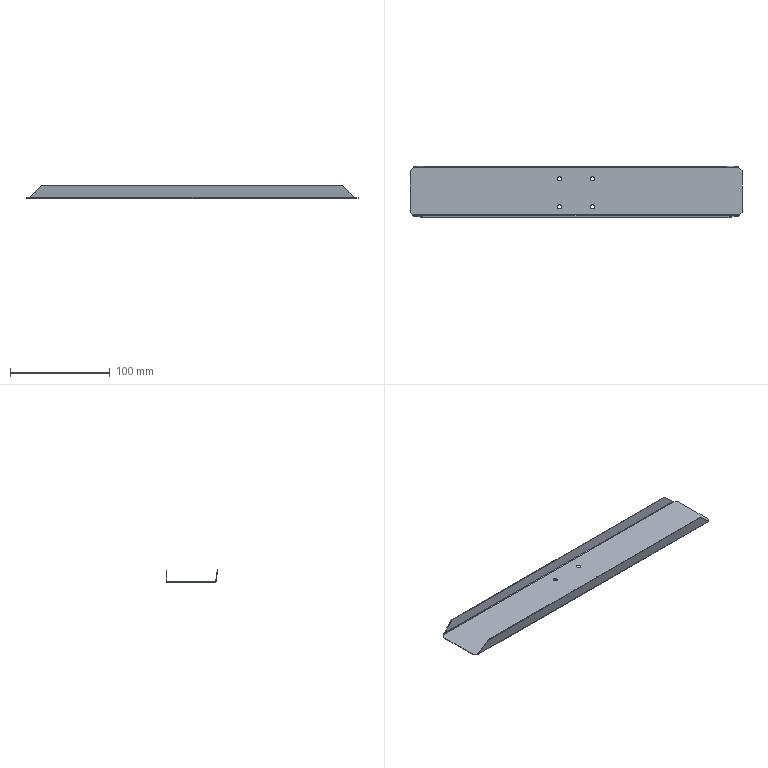Part | SolidWorks | features BaseBody 1 | 1 solid | 34 faces | box 332.2 x 51.676 x 12.864 mm | volume 11858 mm3 | plane 18 | cylinder 12 | spline 4 | commonest cylinder face diameters 4.17 x8 1.5 x2 2.5 x2
STEP:
#1=CARTESIAN_POINT('',(-18.585,-15.223,0.));
#2=VERTEX_POINT('',#1);
#3=CARTESIAN_POINT('',(-14.415,-15.223,0.));
#4=VERTEX_POINT('',#3);
#5=CARTESIAN_POINT('',(-16.5,-15.223,0.));
#6=DIRECTION('',(0.,0.,1.));
#7=DIRECTION('',(-1.,0.,0.));
#8=AXIS2_PLACEMENT_3D('',#5,#6,#7);
#9=CIRCLE('',#8,2.085);
#10=EDGE_CURVE('',#2,#4,#9,.T.);
#11=ORIENTED_EDGE('',*,*,#10,.T.);
#12=CARTESIAN_POINT('',(-14.415,-15.223,-0.5));
#13=VERTEX_POINT('',#12);
#14=CARTESIAN_POINT('',(-14.415,-15.223,0.));
#15=DIRECTION('',(0.,0.,-1.));
#16=VECTOR('',#15,1000.);
#17=LINE('',#14,#16);
#18=EDGE_CURVE('',#4,#13,#17,.T.);
#19=ORIENTED_EDGE('',*,*,#18,.T.);
#20=CARTESIAN_POINT('',(-18.585,-15.223,-0.5));
#21=VERTEX_POINT('',#20);
#22=CARTESIAN_POINT('',(-16.5,-15.223,-0.5));
#23=DIRECTION('',(0.,0.,-1.));
#24=DIRECTION('',(-1.,0.,0.));
#25=AXIS2_PLACEMENT_3D('',#22,#23,#24);
#26=CIRCLE('',#25,2.085);
#27=EDGE_CURVE('',#13,#21,#26,.T.);
#28=ORIENTED_EDGE('',*,*,#27,.T.);
#29=CARTESIAN_POINT('',(-18.585,-15.223,0.));
#30=DIRECTION('',(0.,0.,-1.));
#31=VECTOR('',#30,1000.);
#32=LINE('',#29,#31);
#33=EDGE_CURVE('',#2,#21,#32,.T.);
#34=ORIENTED_EDGE('',*,*,#33,.F.);
#35=EDGE_LOOP('',(#11,#19,#28,#34));
#36=FACE_OUTER_BOUND('',#35,.T.);
#37=CARTESIAN_POINT('',(-16.5,-15.223,0.));
#38=DIRECTION('',(0.,0.,-1.));
#39=DIRECTION('',(-1.,0.,0.));
#40=AXIS2_PLACEMENT_3D('',#37,#38,#39);
#41=CYLINDRICAL_SURFACE('',#40,2.085);
#42=ADVANCED_FACE('',(#36),#41,.F.);
#43=CARTESIAN_POINT('',(14.415,12.777,0.));
#44=VERTEX_POINT('',#43);
#45=CARTESIAN_POINT('',(18.585,12.777,0.));
#46=VERTEX_POINT('',#45);
#47=CARTESIAN_POINT('',(16.5,12.777,0.));
#48=DIRECTION('',(0.,0.,1.));
#49=DIRECTION('',(-1.,0.,0.));
#50=AXIS2_PLACEMENT_3D('',#47,#48,#49);
#51=CIRCLE('',#50,2.085);
#52=EDGE_CURVE('',#44,#46,#51,.T.);
#53=ORIENTED_EDGE('',*,*,#52,.T.);
#54=CARTESIAN_POINT('',(18.585,12.777,-0.5));
#55=VERTEX_POINT('',#54);
#56=CARTESIAN_POINT('',(18.585,12.777,0.));
#57=DIRECTION('',(0.,0.,-1.));
#58=VECTOR('',#57,1000.);
#59=LINE('',#56,#58);
#60=EDGE_CURVE('',#46,#55,#59,.T.);
#61=ORIENTED_EDGE('',*,*,#60,.T.);
#62=CARTESIAN_POINT('',(14.415,12.777,-0.5));
#63=VERTEX_POINT('',#62);
#64=CARTESIAN_POINT('',(16.5,12.777,-0.5));
#65=DIRECTION('',(0.,0.,1.));
#66=DIRECTION('',(-1.,0.,0.));
#67=AXIS2_PLACEMENT_3D('',#64,#65,#66);
#68=CIRCLE('',#67,2.085);
#69=EDGE_CURVE('',#63,#55,#68,.T.);
#70=ORIENTED_EDGE('',*,*,#69,.F.);
#71=CARTESIAN_POINT('',(14.415,12.777,0.));
#72=DIRECTION('',(0.,0.,-1.));
#73=VECTOR('',#72,1000.);
#74=LINE('',#71,#73);
#75=EDGE_CURVE('',#44,#63,#74,.T.);
#76=ORIENTED_EDGE('',*,*,#75,.F.);
#77=EDGE_LOOP('',(#53,#61,#70,#76));
#78=FACE_OUTER_BOUND('',#77,.T.);
#79=CARTESIAN_POINT('',(16.5,12.777,0.));
#80=DIRECTION('',(0.,0.,-1.));
#81=DIRECTION('',(-1.,0.,0.));
#82=AXIS2_PLACEMENT_3D('',#79,#80,#81);
#83=CYLINDRICAL_SURFACE('',#82,2.085);
#84=ADVANCED_FACE('',(#78),#83,.F.);
#85=CARTESIAN_POINT('',(-18.585,12.777,0.));
#86=VERTEX_POINT('',#85);
#87=CARTESIAN_POINT('',(-14.415,12.777,0.));
#88=VERTEX_POINT('',#87);
#89=CARTESIAN_POINT('',(-16.5,12.777,0.));
#90=DIRECTION('',(0.,0.,1.));
#91=DIRECTION('',(-1.,0.,0.));
#92=AXIS2_PLACEMENT_3D('',#89,#90,#91);
#93=CIRCLE('',#92,2.085);
#94=EDGE_CURVE('',#86,#88,#93,.T.);
#95=ORIENTED_EDGE('',*,*,#94,.T.);
#96=CARTESIAN_POINT('',(-14.415,12.777,-0.5));
#97=VERTEX_POINT('',#96);
#98=CARTESIAN_POINT('',(-14.415,12.777,0.));
#99=DIRECTION('',(0.,0.,-1.));
#100=VECTOR('',#99,1000.);
#101=LINE('',#98,#100);
#102=EDGE_CURVE('',#88,#97,#101,.T.);
#103=ORIENTED_EDGE('',*,*,#102,.T.);
#104=CARTESIAN_POINT('',(-18.585,12.777,-0.5));
#105=VERTEX_POINT('',#104);
#106=CARTESIAN_POINT('',(-16.5,12.777,-0.5));
#107=DIRECTION('',(0.,0.,1.));
#108=DIRECTION('',(-1.,0.,0.));
#109=AXIS2_PLACEMENT_3D('',#106,#107,#108);
#110=CIRCLE('',#109,2.085);
#111=EDGE_CURVE('',#105,#97,#110,.T.);
#112=ORIENTED_EDGE('',*,*,#111,.F.);
#113=CARTESIAN_POINT('',(-18.585,12.777,0.));
#114=DIRECTION('',(0.,0.,-1.));
#115=VECTOR('',#114,1000.);
#116=LINE('',#113,#115);
#117=EDGE_CURVE('',#86,#105,#116,.T.);
#118=ORIENTED_EDGE('',*,*,#117,.F.);
#119=EDGE_LOOP('',(#95,#103,#112,#118));
#120=FACE_OUTER_BOUND('',#119,.T.);
#121=CARTESIAN_POINT('',(-16.5,12.777,0.));
#122=DIRECTION('',(0.,0.,-1.));
#123=DIRECTION('',(-1.,0.,0.));
#124=AXIS2_PLACEMENT_3D('',#121,#122,#123);
#125=CYLINDRICAL_SURFACE('',#124,2.085);
#126=ADVANCED_FACE('',(#120),#125,.F.);
#127=CARTESIAN_POINT('',(14.415,-15.223,0.));
#128=VERTEX_POINT('',#127);
#129=CARTESIAN_POINT('',(18.585,-15.223,0.));
#130=VERTEX_POINT('',#129);
#131=CARTESIAN_POINT('',(16.5,-15.223,0.));
#132=DIRECTION('',(0.,0.,1.));
#133=DIRECTION('',(-1.,0.,0.));
#134=AXIS2_PLACEMENT_3D('',#131,#132,#133);
#135=CIRCLE('',#134,2.085);
#136=EDGE_CURVE('',#128,#130,#135,.T.);
#137=ORIENTED_EDGE('',*,*,#136,.T.);
#138=CARTESIAN_POINT('',(18.585,-15.223,-0.5));
#139=VERTEX_POINT('',#138);
#140=CARTESIAN_POINT('',(18.585,-15.223,0.));
#141=DIRECTION('',(0.,0.,-1.));
#142=VECTOR('',#141,1000.);
#143=LINE('',#140,#142);
#144=EDGE_CURVE('',#130,#139,#143,.T.);
#145=ORIENTED_EDGE('',*,*,#144,.T.);
#146=CARTESIAN_POINT('',(14.415,-15.223,-0.5));
#147=VERTEX_POINT('',#146);
#148=CARTESIAN_POINT('',(16.5,-15.223,-0.5));
#149=DIRECTION('',(0.,0.,1.));
#150=DIRECTION('',(-1.,0.,0.));
#151=AXIS2_PLACEMENT_3D('',#148,#149,#150);
#152=CIRCLE('',#151,2.085);
#153=EDGE_CURVE('',#147,#139,#152,.T.);
#154=ORIENTED_EDGE('',*,*,#153,.F.);
#155=CARTESIAN_POINT('',(14.415,-15.223,0.));
#156=DIRECTION('',(0.,0.,-1.));
#157=VECTOR('',#156,1000.);
#158=LINE('',#155,#157);
#159=EDGE_CURVE('',#128,#147,#158,.T.);
#160=ORIENTED_EDGE('',*,*,#159,.F.);
#161=EDGE_LOOP('',(#137,#145,#154,#160));
#162=FACE_OUTER_BOUND('',#161,.T.);
#163=CARTESIAN_POINT('',(16.5,-15.223,0.));
#164=DIRECTION('',(0.,0.,-1.));
#165=DIRECTION('',(-1.,0.,0.));
#166=AXIS2_PLACEMENT_3D('',#163,#164,#165);
#167=CYLINDRICAL_SURFACE('',#166,2.085);
#168=ADVANCED_FACE('',(#162),#167,.F.);
#169=ORIENTED_EDGE('',*,*,#18,.F.);
#170=CARTESIAN_POINT('',(-16.5,-15.223,0.));
#171=DIRECTION('',(0.,0.,1.));
#172=DIRECTION('',(-1.,0.,0.));
#173=AXIS2_PLACEMENT_3D('',#170,#171,#172);
#174=CIRCLE('',#173,2.085);
#175=EDGE_CURVE('',#4,#2,#174,.T.);
#176=ORIENTED_EDGE('',*,*,#175,.T.);
#177=ORIENTED_EDGE('',*,*,#33,.T.);
#178=CARTESIAN_POINT('',(-16.5,-15.223,-0.5));
#179=DIRECTION('',(0.,0.,-1.));
#180=DIRECTION('',(-1.,0.,0.));
#181=AXIS2_PLACEMENT_3D('',#178,#179,#180);
#182=CIRCLE('',#181,2.085);
#183=EDGE_CURVE('',#21,#13,#182,.T.);
#184=ORIENTED_EDGE('',*,*,#183,.T.);
#185=EDGE_LOOP('',(#169,#176,#177,#184));
#186=FACE_OUTER_BOUND('',#185,.T.);
#187=CARTESIAN_POINT('',(-16.5,-15.223,0.));
#188=DIRECTION('',(0.,0.,-1.));
#189=DIRECTION('',(-1.,0.,0.));
#190=AXIS2_PLACEMENT_3D('',#187,#188,#189);
#191=CYLINDRICAL_SURFACE('',#190,2.085);
#192=ADVANCED_FACE('',(#186),#191,.F.);
#193=ORIENTED_EDGE('',*,*,#69,.T.);
#194=CARTESIAN_POINT('',(16.5,12.777,-0.5));
#195=DIRECTION('',(0.,0.,1.));
#196=DIRECTION('',(-1.,0.,0.));
#197=AXIS2_PLACEMENT_3D('',#194,#195,#196);
#198=CIRCLE('',#197,2.085);
#199=EDGE_CURVE('',#55,#63,#198,.T.);
#200=ORIENTED_EDGE('',*,*,#199,.T.);
#201=EDGE_LOOP('',(#193,#200));
#202=FACE_BOUND('',#201,.T.);
#203=ORIENTED_EDGE('',*,*,#111,.T.);
#204=CARTESIAN_POINT('',(-16.5,12.777,-0.5));
#205=DIRECTION('',(0.,0.,1.));
#206=DIRECTION('',(-1.,0.,0.));
#207=AXIS2_PLACEMENT_3D('',#204,#205,#206);
#208=CIRCLE('',#207,2.085);
#209=EDGE_CURVE('',#97,#105,#208,.T.);
#210=ORIENTED_EDGE('',*,*,#209,.T.);
#211=EDGE_LOOP('',(#203,#210));
#212=FACE_BOUND('',#211,.T.);
#213=ORIENTED_EDGE('',*,*,#153,.T.);
#214=CARTESIAN_POINT('',(16.5,-15.223,-0.5));
#215=DIRECTION('',(0.,0.,1.));
#216=DIRECTION('',(-1.,0.,0.));
#217=AXIS2_PLACEMENT_3D('',#214,#215,#216);
#218=CIRCLE('',#217,2.085);
#219=EDGE_CURVE('',#139,#147,#218,.T.);
#220=ORIENTED_EDGE('',*,*,#219,.T.);
#221=EDGE_LOOP('',(#213,#220));
#222=FACE_BOUND('',#221,.T.);
#223=ORIENTED_EDGE('',*,*,#183,.F.);
#224=ORIENTED_EDGE('',*,*,#27,.F.);
#225=EDGE_LOOP('',(#223,#224));
#226=FACE_BOUND('',#225,.T.);
#227=CARTESIAN_POINT('',(166.1,21.,-0.5));
#228=VERTEX_POINT('',#227);
#229=CARTESIAN_POINT('',(166.1,-21.,-0.5));
#230=VERTEX_POINT('',#229);
#231=CARTESIAN_POINT('',(166.1,0.4958,-0.5));
#232=DIRECTION('',(0.,-1.,0.));
#233=VECTOR('',#232,1000.);
#234=LINE('',#231,#233);
#235=EDGE_CURVE('',#228,#230,#234,.T.);
#236=ORIENTED_EDGE('',*,*,#235,.T.);
#237=CARTESIAN_POINT('',(163.877,-23.223,-0.5));
#238=VERTEX_POINT('',#237);
#239=CARTESIAN_POINT('',(166.1,-21.,-0.5));
#240=DIRECTION('',(-0.7071,-0.7071,0.));
#241=VECTOR('',#240,1000.);
#242=LINE('',#239,#241);
#243=EDGE_CURVE('',#230,#238,#242,.T.);
#244=ORIENTED_EDGE('',*,*,#243,.T.);
#245=CARTESIAN_POINT('',(-163.877,-23.223,-0.5));
#246=VERTEX_POINT('',#245);
#247=CARTESIAN_POINT('',(0.,-23.223,-0.5));
#248=DIRECTION('',(-1.,0.,0.));
#249=VECTOR('',#248,1000.);
#250=LINE('',#247,#249);
#251=EDGE_CURVE('',#238,#246,#250,.T.);
#252=ORIENTED_EDGE('',*,*,#251,.T.);
#253=CARTESIAN_POINT('',(-166.1,-21.,-0.5));
#254=VERTEX_POINT('',#253);
#255=CARTESIAN_POINT('',(-163.877,-23.223,-0.5));
#256=DIRECTION('',(-0.7071,0.7071,0.));
#257=VECTOR('',#256,1000.);
#258=LINE('',#255,#257);
#259=EDGE_CURVE('',#246,#254,#258,.T.);
#260=ORIENTED_EDGE('',*,*,#259,.T.);
#261=CARTESIAN_POINT('',(-166.1,21.,-0.5));
#262=VERTEX_POINT('',#261);
#263=CARTESIAN_POINT('',(-166.1,0.4958,-0.5));
#264=DIRECTION('',(0.,1.,0.));
#265=VECTOR('',#264,1000.);
#266=LINE('',#263,#265);
#267=EDGE_CURVE('',#254,#262,#266,.T.);
#268=ORIENTED_EDGE('',*,*,#267,.T.);
#269=CARTESIAN_POINT('',(-162.885,24.215,-0.5));
#270=VERTEX_POINT('',#269);
#271=CARTESIAN_POINT('',(-166.1,21.,-0.5));
#272=DIRECTION('',(0.7071,0.7071,0.));
#273=VECTOR('',#272,1000.);
#274=LINE('',#271,#273);
#275=EDGE_CURVE('',#262,#270,#274,.T.);
#276=ORIENTED_EDGE('',*,*,#275,.T.);
#277=CARTESIAN_POINT('',(162.885,24.215,-0.5));
#278=VERTEX_POINT('',#277);
#279=CARTESIAN_POINT('',(0.,24.215,-0.5));
#280=DIRECTION('',(1.,0.,0.));
#281=VECTOR('',#280,1000.);
#282=LINE('',#279,#281);
#283=EDGE_CURVE('',#270,#278,#282,.T.);
#284=ORIENTED_EDGE('',*,*,#283,.T.);
#285=CARTESIAN_POINT('',(162.885,24.215,-0.5));
#286=DIRECTION('',(0.7071,-0.7071,0.));
#287=VECTOR('',#286,1000.);
#288=LINE('',#285,#287);
#289=EDGE_CURVE('',#278,#228,#288,.T.);
#290=ORIENTED_EDGE('',*,*,#289,.T.);
#291=EDGE_LOOP('',(#236,#244,#252,#260,#268,#276,#284,#290));
#292=FACE_OUTER_BOUND('',#291,.T.);
#293=CARTESIAN_POINT('',(166.1,-23.223,-0.5));
#294=DIRECTION('',(0.,0.,-1.));
#295=DIRECTION('',(-1.,0.,0.));
#296=AXIS2_PLACEMENT_3D('',#293,#294,#295);
#297=PLANE('',#296);
#298=ADVANCED_FACE('',(#202,#212,#222,#226,#292),#297,.T.);
#299=ORIENTED_EDGE('',*,*,#52,.F.);
#300=CARTESIAN_POINT('',(16.5,12.777,0.));
#301=DIRECTION('',(0.,0.,1.));
#302=DIRECTION('',(-1.,0.,0.));
#303=AXIS2_PLACEMENT_3D('',#300,#301,#302);
#304=CIRCLE('',#303,2.085);
#305=EDGE_CURVE('',#46,#44,#304,.T.);
#306=ORIENTED_EDGE('',*,*,#305,.F.);
#307=EDGE_LOOP('',(#299,#306));
#308=FACE_BOUND('',#307,.T.);
#309=ORIENTED_EDGE('',*,*,#94,.F.);
#310=CARTESIAN_POINT('',(-16.5,12.777,0.));
#311=DIRECTION('',(0.,0.,1.));
#312=DIRECTION('',(-1.,0.,0.));
#313=AXIS2_PLACEMENT_3D('',#310,#311,#312);
#314=CIRCLE('',#313,2.085);
#315=EDGE_CURVE('',#88,#86,#314,.T.);
#316=ORIENTED_EDGE('',*,*,#315,.F.);
#317=EDGE_LOOP('',(#309,#316));
#318=FACE_BOUND('',#317,.T.);
#319=ORIENTED_EDGE('',*,*,#136,.F.);
#320=CARTESIAN_POINT('',(16.5,-15.223,0.));
#321=DIRECTION('',(0.,0.,1.));
#322=DIRECTION('',(-1.,0.,0.));
#323=AXIS2_PLACEMENT_3D('',#320,#321,#322);
#324=CIRCLE('',#323,2.085);
#325=EDGE_CURVE('',#130,#128,#324,.T.);
#326=ORIENTED_EDGE('',*,*,#325,.F.);
#327=EDGE_LOOP('',(#319,#326));
#328=FACE_BOUND('',#327,.T.);
#329=ORIENTED_EDGE('',*,*,#10,.F.);
#330=ORIENTED_EDGE('',*,*,#175,.F.);
#331=EDGE_LOOP('',(#329,#330));
#332=FACE_BOUND('',#331,.T.);
#333=CARTESIAN_POINT('',(163.877,-23.223,0.));
#334=VERTEX_POINT('',#333);
#335=CARTESIAN_POINT('',(-163.877,-23.223,0.));
#336=VERTEX_POINT('',#335);
#337=CARTESIAN_POINT('',(0.,-23.223,0.));
#338=DIRECTION('',(-1.,0.,0.));
#339=VECTOR('',#338,1000.);
#340=LINE('',#337,#339);
#341=EDGE_CURVE('',#334,#336,#340,.T.);
#342=ORIENTED_EDGE('',*,*,#341,.F.);
#343=CARTESIAN_POINT('',(166.1,-21.,0.));
#344=VERTEX_POINT('',#343);
#345=CARTESIAN_POINT('',(163.877,-23.223,0.));
#346=DIRECTION('',(-0.7071,-0.7071,0.));
#347=VECTOR('',#346,1000.);
#348=LINE('',#345,#347);
#349=EDGE_CURVE('',#344,#334,#348,.T.);
#350=ORIENTED_EDGE('',*,*,#349,.F.);
#351=CARTESIAN_POINT('',(166.1,21.,0.));
#352=VERTEX_POINT('',#351);
#353=CARTESIAN_POINT('',(166.1,0.4958,0.));
#354=DIRECTION('',(0.,-1.,0.));
#355=VECTOR('',#354,1000.);
#356=LINE('',#353,#355);
#357=EDGE_CURVE('',#352,#344,#356,.T.);
#358=ORIENTED_EDGE('',*,*,#357,.F.);
#359=CARTESIAN_POINT('',(162.885,24.215,0.));
#360=VERTEX_POINT('',#359);
#361=CARTESIAN_POINT('',(166.1,21.,0.));
#362=DIRECTION('',(0.7071,-0.7071,0.));
#363=VECTOR('',#362,1000.);
#364=LINE('',#361,#363);
#365=EDGE_CURVE('',#360,#352,#364,.T.);
#366=ORIENTED_EDGE('',*,*,#365,.F.);
#367=CARTESIAN_POINT('',(-162.885,24.215,0.));
#368=VERTEX_POINT('',#367);
#369=CARTESIAN_POINT('',(0.,24.215,0.));
#370=DIRECTION('',(1.,0.,0.));
#371=VECTOR('',#370,1000.);
#372=LINE('',#369,#371);
#373=EDGE_CURVE('',#368,#360,#372,.T.);
#374=ORIENTED_EDGE('',*,*,#373,.F.);
#375=CARTESIAN_POINT('',(-166.1,21.,0.));
#376=VERTEX_POINT('',#375);
#377=CARTESIAN_POINT('',(-162.885,24.215,0.));
#378=DIRECTION('',(0.7071,0.7071,0.));
#379=VECTOR('',#378,1000.);
#380=LINE('',#377,#379);
#381=EDGE_CURVE('',#376,#368,#380,.T.);
#382=ORIENTED_EDGE('',*,*,#381,.F.);
#383=CARTESIAN_POINT('',(-166.1,-21.,0.));
#384=VERTEX_POINT('',#383);
#385=CARTESIAN_POINT('',(-166.1,0.4958,0.));
#386=DIRECTION('',(0.,1.,0.));
#387=VECTOR('',#386,1000.);
#388=LINE('',#385,#387);
#389=EDGE_CURVE('',#384,#376,#388,.T.);
#390=ORIENTED_EDGE('',*,*,#389,.F.);
#391=CARTESIAN_POINT('',(-166.1,-21.,0.));
#392=DIRECTION('',(-0.7071,0.7071,0.));
#393=VECTOR('',#392,1000.);
#394=LINE('',#391,#393);
#395=EDGE_CURVE('',#336,#384,#394,.T.);
#396=ORIENTED_EDGE('',*,*,#395,.F.);
#397=EDGE_LOOP('',(#342,#350,#358,#366,#374,#382,#390,#396));
#398=FACE_OUTER_BOUND('',#397,.T.);
#399=CARTESIAN_POINT('',(166.1,-23.223,0.));
#400=DIRECTION('',(0.,0.,-1.));
#401=DIRECTION('',(-1.,0.,0.));
#402=AXIS2_PLACEMENT_3D('',#399,#400,#401);
#403=PLANE('',#402);
#404=ADVANCED_FACE('',(#308,#318,#328,#332,#398),#403,.F.);
#405=ORIENTED_EDGE('',*,*,#60,.F.);
#406=ORIENTED_EDGE('',*,*,#305,.T.);
#407=ORIENTED_EDGE('',*,*,#75,.T.);
#408=ORIENTED_EDGE('',*,*,#199,.F.);
#409=EDGE_LOOP('',(#405,#406,#407,#408));
#410=FACE_OUTER_BOUND('',#409,.T.);
#411=CARTESIAN_POINT('',(16.5,12.777,0.));
#412=DIRECTION('',(0.,0.,-1.));
#413=DIRECTION('',(-1.,0.,0.));
#414=AXIS2_PLACEMENT_3D('',#411,#412,#413);
#415=CYLINDRICAL_SURFACE('',#414,2.085);
#416=ADVANCED_FACE('',(#410),#415,.F.);
#417=ORIENTED_EDGE('',*,*,#102,.F.);
#418=ORIENTED_EDGE('',*,*,#315,.T.);
#419=ORIENTED_EDGE('',*,*,#117,.T.);
#420=ORIENTED_EDGE('',*,*,#209,.F.);
#421=EDGE_LOOP('',(#417,#418,#419,#420));
#422=FACE_OUTER_BOUND('',#421,.T.);
#423=CARTESIAN_POINT('',(-16.5,12.777,0.));
#424=DIRECTION('',(0.,0.,-1.));
#425=DIRECTION('',(-1.,0.,0.));
#426=AXIS2_PLACEMENT_3D('',#423,#424,#425);
#427=CYLINDRICAL_SURFACE('',#426,2.085);
#428=ADVANCED_FACE('',(#422),#427,.F.);
#429=ORIENTED_EDGE('',*,*,#144,.F.);
#430=ORIENTED_EDGE('',*,*,#325,.T.);
#431=ORIENTED_EDGE('',*,*,#159,.T.);
#432=ORIENTED_EDGE('',*,*,#219,.F.);
#433=EDGE_LOOP('',(#429,#430,#431,#432));
#434=FACE_OUTER_BOUND('',#433,.T.);
#435=CARTESIAN_POINT('',(16.5,-15.223,0.));
#436=DIRECTION('',(0.,0.,-1.));
#437=DIRECTION('',(-1.,0.,0.));
#438=AXIS2_PLACEMENT_3D('',#435,#436,#437);
#439=CYLINDRICAL_SURFACE('',#438,2.085);
#440=ADVANCED_FACE('',(#434),#439,.F.);
#441=CARTESIAN_POINT('',(166.1,-21.,-0.25));
#442=DIRECTION('',(0.,0.,1.));
#443=VECTOR('',#442,1000.);
#444=LINE('',#441,#443);
#445=EDGE_CURVE('',#230,#344,#444,.T.);
#446=ORIENTED_EDGE('',*,*,#445,.T.);
#447=ORIENTED_EDGE('',*,*,#349,.T.);
#448=CARTESIAN_POINT('',(163.877,-23.223,-0.25));
#449=DIRECTION('',(0.,0.,1.));
#450=VECTOR('',#449,1000.);
#451=LINE('',#448,#450);
#452=EDGE_CURVE('',#238,#334,#451,.T.);
#453=ORIENTED_EDGE('',*,*,#452,.F.);
#454=ORIENTED_EDGE('',*,*,#243,.F.);
#455=EDGE_LOOP('',(#446,#447,#453,#454));
#456=FACE_OUTER_BOUND('',#455,.T.);
#457=CARTESIAN_POINT('',(163.877,-23.223,-0.5));
#458=DIRECTION('',(0.7071,-0.7071,0.));
#459=DIRECTION('',(0.7071,0.7071,0.));
#460=AXIS2_PLACEMENT_3D('',#457,#458,#459);
#461=PLANE('',#460);
#462=ADVANCED_FACE('',(#456),#461,.T.);
#463=ORIENTED_EDGE('',*,*,#235,.F.);
#464=CARTESIAN_POINT('',(166.1,21.,-0.25));
#465=DIRECTION('',(0.,0.,1.));
#466=VECTOR('',#465,1000.);
#467=LINE('',#464,#466);
#468=EDGE_CURVE('',#228,#352,#467,.T.);
#469=ORIENTED_EDGE('',*,*,#468,.T.);
#470=ORIENTED_EDGE('',*,*,#357,.T.);
#471=ORIENTED_EDGE('',*,*,#445,.F.);
#472=EDGE_LOOP('',(#463,#469,#470,#471));
#473=FACE_OUTER_BOUND('',#472,.T.);
#474=CARTESIAN_POINT('',(166.1,-21.,-0.5));
#475=DIRECTION('',(1.,0.,0.));
#476=DIRECTION('',(0.,1.,0.));
#477=AXIS2_PLACEMENT_3D('',#474,#475,#476);
#478=PLANE('',#477);
#479=ADVANCED_FACE('',(#473),#478,.T.);
#480=ORIENTED_EDGE('',*,*,#365,.T.);
#481=ORIENTED_EDGE('',*,*,#468,.F.);
#482=ORIENTED_EDGE('',*,*,#289,.F.);
#483=CARTESIAN_POINT('',(162.885,24.215,-0.25));
#484=DIRECTION('',(0.,0.,-1.));
#485=VECTOR('',#484,1000.);
#486=LINE('',#483,#485);
#487=EDGE_CURVE('',#360,#278,#486,.T.);
#488=ORIENTED_EDGE('',*,*,#487,.F.);
#489=EDGE_LOOP('',(#480,#481,#482,#488));
#490=FACE_OUTER_BOUND('',#489,.T.);
#491=CARTESIAN_POINT('',(166.1,21.,-0.5));
#492=DIRECTION('',(0.7071,0.7071,0.));
#493=DIRECTION('',(-0.7071,0.7071,0.));
#494=AXIS2_PLACEMENT_3D('',#491,#492,#493);
#495=PLANE('',#494);
#496=ADVANCED_FACE('',(#490),#495,.T.);
#497=CARTESIAN_POINT('',(161.315,25.465,0.75));
#498=VERTEX_POINT('',#497);
#499=CARTESIAN_POINT('',(162.885,24.215,-0.5));
#500=CARTESIAN_POINT('',(162.753,24.38,-0.5));
#501=CARTESIAN_POINT('',(162.625,24.54,-0.4679));
#502=CARTESIAN_POINT('',(162.362,24.844,-0.3424));
#503=CARTESIAN_POINT('',(162.232,24.982,-0.2505));
#504=CARTESIAN_POINT('',(161.97,25.213,-0.01937));
#505=CARTESIAN_POINT('',(161.839,25.306,0.1193));
#506=CARTESIAN_POINT('',(161.578,25.431,0.4205));
#507=CARTESIAN_POINT('',(161.447,25.465,0.585));
#508=CARTESIAN_POINT('',(161.315,25.465,0.75));
#509=B_SPLINE_CURVE_WITH_KNOTS('',3,(#499,#500,#501,#502,#503,#504,#505,#506,#507,#508),.UNSPECIFIED.,.F.,.F.,(4,2,2,2,4),(0.,0.000625,0.00125,0.001875,0.0025),.UNSPECIFIED.);
#510=EDGE_CURVE('',#278,#498,#509,.T.);
#511=ORIENTED_EDGE('',*,*,#510,.F.);
#512=ORIENTED_EDGE('',*,*,#283,.F.);
#513=CARTESIAN_POINT('',(-161.315,25.465,0.75));
#514=VERTEX_POINT('',#513);
#515=CARTESIAN_POINT('',(-161.315,25.465,0.75));
#516=CARTESIAN_POINT('',(-161.447,25.465,0.585));
#517=CARTESIAN_POINT('',(-161.575,25.433,0.4242));
#518=CARTESIAN_POINT('',(-161.838,25.307,0.1206));
#519=CARTESIAN_POINT('',(-161.968,25.215,-0.01703));
#520=CARTESIAN_POINT('',(-162.23,24.984,-0.2487));
#521=CARTESIAN_POINT('',(-162.361,24.845,-0.3415));
#522=CARTESIAN_POINT('',(-162.622,24.544,-0.4668));
#523=CARTESIAN_POINT('',(-162.753,24.38,-0.5));
#524=CARTESIAN_POINT('',(-162.885,24.215,-0.5));
#525=B_SPLINE_CURVE_WITH_KNOTS('',3,(#515,#516,#517,#518,#519,#520,#521,#522,#523,#524),.UNSPECIFIED.,.F.,.F.,(4,2,2,2,4),(0.,0.000625,0.00125,0.001875,0.0025),.UNSPECIFIED.);
#526=EDGE_CURVE('',#514,#270,#525,.T.);
#527=ORIENTED_EDGE('',*,*,#526,.F.);
#528=CARTESIAN_POINT('',(0.,25.465,0.75));
#529=DIRECTION('',(-1.,0.,0.));
#530=VECTOR('',#529,1000.);
#531=LINE('',#528,#530);
#532=EDGE_CURVE('',#498,#514,#531,.T.);
#533=ORIENTED_EDGE('',*,*,#532,.F.);
#534=EDGE_LOOP('',(#511,#512,#527,#533));
#535=FACE_OUTER_BOUND('',#534,.T.);
#536=CARTESIAN_POINT('',(-164.84,24.215,0.75));
#537=DIRECTION('',(1.,0.,0.));
#538=DIRECTION('',(0.,1.,0.));
#539=AXIS2_PLACEMENT_3D('',#536,#537,#538);
#540=CYLINDRICAL_SURFACE('',#539,1.25);
#541=ADVANCED_FACE('',(#535),#540,.T.);
#542=ORIENTED_EDGE('',*,*,#275,.F.);
#543=CARTESIAN_POINT('',(-166.1,21.,-0.25));
#544=DIRECTION('',(0.,0.,1.));
#545=VECTOR('',#544,1000.);
#546=LINE('',#543,#545);
#547=EDGE_CURVE('',#262,#376,#546,.T.);
#548=ORIENTED_EDGE('',*,*,#547,.T.);
#549=ORIENTED_EDGE('',*,*,#381,.T.);
#550=CARTESIAN_POINT('',(-162.885,24.215,-0.25));
#551=DIRECTION('',(0.,0.,-1.));
#552=VECTOR('',#551,1000.);
#553=LINE('',#550,#552);
#554=EDGE_CURVE('',#368,#270,#553,.T.);
#555=ORIENTED_EDGE('',*,*,#554,.T.);
#556=EDGE_LOOP('',(#542,#548,#549,#555));
#557=FACE_OUTER_BOUND('',#556,.T.);
#558=CARTESIAN_POINT('',(-162.885,24.215,-0.5));
#559=DIRECTION('',(-0.7071,0.7071,0.));
#560=DIRECTION('',(-0.7071,-0.7071,0.));
#561=AXIS2_PLACEMENT_3D('',#558,#559,#560);
#562=PLANE('',#561);
#563=ADVANCED_FACE('',(#557),#562,.T.);
#564=ORIENTED_EDGE('',*,*,#267,.F.);
#565=CARTESIAN_POINT('',(-166.1,-21.,-0.25));
#566=DIRECTION('',(0.,0.,1.));
#567=VECTOR('',#566,1000.);
#568=LINE('',#565,#567);
#569=EDGE_CURVE('',#254,#384,#568,.T.);
#570=ORIENTED_EDGE('',*,*,#569,.T.);
#571=ORIENTED_EDGE('',*,*,#389,.T.);
#572=ORIENTED_EDGE('',*,*,#547,.F.);
#573=EDGE_LOOP('',(#564,#570,#571,#572));
#574=FACE_OUTER_BOUND('',#573,.T.);
#575=CARTESIAN_POINT('',(-166.1,-21.,-0.5));
#576=DIRECTION('',(-1.,0.,0.));
#577=DIRECTION('',(0.,0.,1.));
#578=AXIS2_PLACEMENT_3D('',#575,#576,#577);
#579=PLANE('',#578);
#580=ADVANCED_FACE('',(#574),#579,.T.);
#581=ORIENTED_EDGE('',*,*,#569,.F.);
#582=ORIENTED_EDGE('',*,*,#259,.F.);
#583=CARTESIAN_POINT('',(-163.877,-23.223,-0.25));
#584=DIRECTION('',(0.,0.,-1.));
#585=VECTOR('',#584,1000.);
#586=LINE('',#583,#585);
#587=EDGE_CURVE('',#336,#246,#586,.T.);
#588=ORIENTED_EDGE('',*,*,#587,.F.);
#589=ORIENTED_EDGE('',*,*,#395,.T.);
#590=EDGE_LOOP('',(#581,#582,#588,#589));
#591=FACE_OUTER_BOUND('',#590,.T.);
#592=CARTESIAN_POINT('',(-166.1,-21.,-0.5));
#593=DIRECTION('',(-0.7071,-0.7071,0.));
#594=DIRECTION('',(0.7071,-0.7071,0.));
#595=AXIS2_PLACEMENT_3D('',#592,#593,#594);
#596=PLANE('',#595);
#597=ADVANCED_FACE('',(#591),#596,.T.);
#598=CARTESIAN_POINT('',(162.455,-24.459,0.5652));
#599=VERTEX_POINT('',#598);
#600=CARTESIAN_POINT('',(162.455,-24.459,0.5652));
#601=CARTESIAN_POINT('',(162.574,-24.437,0.4174));
#602=CARTESIAN_POINT('',(162.691,-24.389,0.2769));
#603=CARTESIAN_POINT('',(162.928,-24.246,0.01725));
#604=CARTESIAN_POINT('',(163.047,-24.151,-0.09991));
#605=CARTESIAN_POINT('',(163.283,-23.928,-0.2927));
#606=CARTESIAN_POINT('',(163.403,-23.797,-0.3701));
#607=CARTESIAN_POINT('',(163.639,-23.521,-0.4729));
#608=CARTESIAN_POINT('',(163.757,-23.372,-0.5));
#609=CARTESIAN_POINT('',(163.877,-23.223,-0.5));
#610=B_SPLINE_CURVE_WITH_KNOTS('',3,(#600,#601,#602,#603,#604,#605,#606,#607,#608,#609),.UNSPECIFIED.,.F.,.F.,(4,2,2,2,4),(0.,0.0005661,0.001132,0.001698,0.002265),.UNSPECIFIED.);
#611=EDGE_CURVE('',#599,#238,#610,.T.);
#612=ORIENTED_EDGE('',*,*,#611,.F.);
#613=CARTESIAN_POINT('',(-162.455,-24.459,0.5652));
#614=VERTEX_POINT('',#613);
#615=CARTESIAN_POINT('',(0.,-24.459,0.5652));
#616=DIRECTION('',(1.,0.,0.));
#617=VECTOR('',#616,1000.);
#618=LINE('',#615,#617);
#619=EDGE_CURVE('',#614,#599,#618,.T.);
#620=ORIENTED_EDGE('',*,*,#619,.F.);
#621=CARTESIAN_POINT('',(-163.877,-23.223,-0.5));
#622=CARTESIAN_POINT('',(-163.757,-23.372,-0.5));
#623=CARTESIAN_POINT('',(-163.641,-23.518,-0.4736));
#624=CARTESIAN_POINT('',(-163.404,-23.796,-0.3706));
#625=CARTESIAN_POINT('',(-163.285,-23.926,-0.2938));
#626=CARTESIAN_POINT('',(-163.049,-24.15,-0.1014));
#627=CARTESIAN_POINT('',(-162.929,-24.246,0.01658));
#628=CARTESIAN_POINT('',(-162.693,-24.388,0.2746));
#629=CARTESIAN_POINT('',(-162.574,-24.437,0.4174));
#630=CARTESIAN_POINT('',(-162.455,-24.459,0.5652));
#631=B_SPLINE_CURVE_WITH_KNOTS('',3,(#621,#622,#623,#624,#625,#626,#627,#628,#629,#630),.UNSPECIFIED.,.F.,.F.,(4,2,2,2,4),(0.,0.0005661,0.001132,0.001698,0.002265),.UNSPECIFIED.);
#632=EDGE_CURVE('',#246,#614,#631,.T.);
#633=ORIENTED_EDGE('',*,*,#632,.F.);
#634=ORIENTED_EDGE('',*,*,#251,.F.);
#635=EDGE_LOOP('',(#612,#620,#633,#634));
#636=FACE_OUTER_BOUND('',#635,.T.);
#637=CARTESIAN_POINT('',(165.844,-23.223,0.75));
#638=DIRECTION('',(-1.,0.,0.));
#639=DIRECTION('',(0.,0.,1.));
#640=AXIS2_PLACEMENT_3D('',#637,#638,#639);
#641=CYLINDRICAL_SURFACE('',#640,1.25);
#642=ADVANCED_FACE('',(#636),#641,.T.);
#643=CARTESIAN_POINT('',(-162.455,-23.965,0.6391));
#644=VERTEX_POINT('',#643);
#645=CARTESIAN_POINT('',(162.455,-23.965,0.6391));
#646=VERTEX_POINT('',#645);
#647=CARTESIAN_POINT('',(0.,-23.965,0.6391));
#648=DIRECTION('',(1.,0.,0.));
#649=VECTOR('',#648,1000.);
#650=LINE('',#647,#649);
#651=EDGE_CURVE('',#644,#646,#650,.T.);
#652=ORIENTED_EDGE('',*,*,#651,.T.);
#653=CARTESIAN_POINT('',(162.455,-23.965,0.6391));
#654=CARTESIAN_POINT('',(162.574,-23.951,0.5505));
#655=CARTESIAN_POINT('',(162.691,-23.923,0.4658));
#656=CARTESIAN_POINT('',(162.927,-23.837,0.3109));
#657=CARTESIAN_POINT('',(163.047,-23.78,0.24));
#658=CARTESIAN_POINT('',(163.402,-23.579,0.06628));
#659=CARTESIAN_POINT('',(163.638,-23.402,0.000000007));
#660=CARTESIAN_POINT('',(163.877,-23.223,0.));
#661=B_SPLINE_CURVE_WITH_KNOTS('',3,(#653,#654,#655,#656,#657,#658,#659,#660),.UNSPECIFIED.,.F.,.F.,(4,2,2,4),(0.,0.0004418,0.0008836,0.001767),.UNSPECIFIED.);
#662=EDGE_CURVE('',#646,#334,#661,.T.);
#663=ORIENTED_EDGE('',*,*,#662,.T.);
#664=ORIENTED_EDGE('',*,*,#341,.T.);
#665=CARTESIAN_POINT('',(-163.877,-23.223,0.));
#666=CARTESIAN_POINT('',(-163.758,-23.313,0.000000004));
#667=CARTESIAN_POINT('',(-163.64,-23.401,0.01599));
#668=CARTESIAN_POINT('',(-163.404,-23.566,0.07744));
#669=CARTESIAN_POINT('',(-163.285,-23.645,0.1237));
#670=CARTESIAN_POINT('',(-162.93,-23.847,0.2972));
#671=CARTESIAN_POINT('',(-162.694,-23.938,0.4619));
#672=CARTESIAN_POINT('',(-162.455,-23.965,0.6391));
#673=B_SPLINE_CURVE_WITH_KNOTS('',3,(#665,#666,#667,#668,#669,#670,#671,#672),.UNSPECIFIED.,.F.,.F.,(4,2,2,4),(0.,0.0004418,0.0008836,0.001767),.UNSPECIFIED.);
#674=EDGE_CURVE('',#336,#644,#673,.T.);
#675=ORIENTED_EDGE('',*,*,#674,.T.);
#676=EDGE_LOOP('',(#652,#663,#664,#675));
#677=FACE_OUTER_BOUND('',#676,.T.);
#678=CARTESIAN_POINT('',(165.844,-23.223,0.75));
#679=DIRECTION('',(-1.,0.,0.));
#680=DIRECTION('',(0.,0.,1.));
#681=AXIS2_PLACEMENT_3D('',#678,#679,#680);
#682=CYLINDRICAL_SURFACE('',#681,0.75);
#683=ADVANCED_FACE('',(#677),#682,.F.);
#684=ORIENTED_EDGE('',*,*,#373,.T.);
#685=CARTESIAN_POINT('',(161.315,24.965,0.75));
#686=VERTEX_POINT('',#685);
#687=CARTESIAN_POINT('',(162.885,24.215,0.));
#688=CARTESIAN_POINT('',(162.753,24.314,0.));
#689=CARTESIAN_POINT('',(162.624,24.411,0.01949));
#690=CARTESIAN_POINT('',(162.363,24.591,0.09421));
#691=CARTESIAN_POINT('',(162.231,24.676,0.1504));
#692=CARTESIAN_POINT('',(161.97,24.814,0.2884));
#693=CARTESIAN_POINT('',(161.84,24.869,0.3713));
#694=CARTESIAN_POINT('',(161.577,24.945,0.5535));
#695=CARTESIAN_POINT('',(161.447,24.965,0.651));
#696=CARTESIAN_POINT('',(161.315,24.965,0.75));
#697=B_SPLINE_CURVE_WITH_KNOTS('',3,(#687,#688,#689,#690,#691,#692,#693,#694,#695,#696),.UNSPECIFIED.,.F.,.F.,(4,2,2,2,4),(0.,0.0004881,0.0009761,0.001464,0.001952),.UNSPECIFIED.);
#698=EDGE_CURVE('',#360,#686,#697,.T.);
#699=ORIENTED_EDGE('',*,*,#698,.T.);
#700=CARTESIAN_POINT('',(-161.315,24.965,0.75));
#701=VERTEX_POINT('',#700);
#702=CARTESIAN_POINT('',(0.,24.965,0.75));
#703=DIRECTION('',(-1.,0.,0.));
#704=VECTOR('',#703,1000.);
#705=LINE('',#702,#704);
#706=EDGE_CURVE('',#686,#701,#705,.T.);
#707=ORIENTED_EDGE('',*,*,#706,.T.);
#708=CARTESIAN_POINT('',(-161.315,24.965,0.75));
#709=CARTESIAN_POINT('',(-161.447,24.965,0.651));
#710=CARTESIAN_POINT('',(-161.576,24.945,0.554));
#711=CARTESIAN_POINT('',(-161.837,24.87,0.3732));
#712=CARTESIAN_POINT('',(-161.969,24.814,0.289));
#713=CARTESIAN_POINT('',(-162.23,24.676,0.1508));
#714=CARTESIAN_POINT('',(-162.36,24.593,0.09517));
#715=CARTESIAN_POINT('',(-162.623,24.411,0.01949));
#716=CARTESIAN_POINT('',(-162.753,24.314,0.));
#717=CARTESIAN_POINT('',(-162.885,24.215,0.));
#718=B_SPLINE_CURVE_WITH_KNOTS('',3,(#708,#709,#710,#711,#712,#713,#714,#715,#716,#717),.UNSPECIFIED.,.F.,.F.,(4,2,2,2,4),(0.,0.0004881,0.0009761,0.001464,0.001952),.UNSPECIFIED.);
#719=EDGE_CURVE('',#701,#368,#718,.T.);
#720=ORIENTED_EDGE('',*,*,#719,.T.);
#721=EDGE_LOOP('',(#684,#699,#707,#720));
#722=FACE_OUTER_BOUND('',#721,.T.);
#723=CARTESIAN_POINT('',(-164.84,24.215,0.75));
#724=DIRECTION('',(1.,0.,0.));
#725=DIRECTION('',(0.,1.,0.));
#726=AXIS2_PLACEMENT_3D('',#723,#724,#725);
#727=CYLINDRICAL_SURFACE('',#726,0.75);
#728=ADVANCED_FACE('',(#722),#727,.F.);
#729=CARTESIAN_POINT('',(-150.6,25.465,11.465));
#730=VERTEX_POINT('',#729);
#731=CARTESIAN_POINT('',(150.6,25.465,11.465));
#732=VERTEX_POINT('',#731);
#733=CARTESIAN_POINT('',(0.,25.465,11.465));
#734=DIRECTION('',(1.,0.,0.));
#735=VECTOR('',#734,1000.);
#736=LINE('',#733,#735);
#737=EDGE_CURVE('',#730,#732,#736,.T.);
#738=ORIENTED_EDGE('',*,*,#737,.T.);
#739=CARTESIAN_POINT('',(150.6,25.465,11.465));
#740=DIRECTION('',(0.7071,0.,-0.7071));
#741=VECTOR('',#740,1000.);
#742=LINE('',#739,#741);
#743=EDGE_CURVE('',#732,#498,#742,.T.);
#744=ORIENTED_EDGE('',*,*,#743,.T.);
#745=ORIENTED_EDGE('',*,*,#532,.T.);
#746=CARTESIAN_POINT('',(-161.315,25.465,0.75));
#747=DIRECTION('',(0.7071,0.,0.7071));
#748=VECTOR('',#747,1000.);
#749=LINE('',#746,#748);
#750=EDGE_CURVE('',#514,#730,#749,.T.);
#751=ORIENTED_EDGE('',*,*,#750,.T.);
#752=EDGE_LOOP('',(#738,#744,#745,#751));
#753=FACE_OUTER_BOUND('',#752,.T.);
#754=CARTESIAN_POINT('',(163.25,25.465,0.75));
#755=DIRECTION('',(0.,1.,0.));
#756=DIRECTION('',(-1.,0.,0.));
#757=AXIS2_PLACEMENT_3D('',#754,#755,#756);
#758=PLANE('',#757);
#759=ADVANCED_FACE('',(#753),#758,.T.);
#760=ORIENTED_EDGE('',*,*,#510,.T.);
#761=CARTESIAN_POINT('',(161.315,25.215,0.75));
#762=DIRECTION('',(0.,-1.,0.));
#763=VECTOR('',#762,1000.);
#764=LINE('',#761,#763);
#765=EDGE_CURVE('',#498,#686,#764,.T.);
#766=ORIENTED_EDGE('',*,*,#765,.T.);
#767=ORIENTED_EDGE('',*,*,#698,.F.);
#768=ORIENTED_EDGE('',*,*,#487,.T.);
#769=EDGE_LOOP('',(#760,#766,#767,#768));
#770=FACE_OUTER_BOUND('',#769,.T.);
#771=CARTESIAN_POINT('',(161.315,25.47,0.75));
#772=CARTESIAN_POINT('',(161.446,25.47,0.5857));
#773=CARTESIAN_POINT('',(161.576,25.437,0.4215));
#774=CARTESIAN_POINT('',(161.838,25.311,0.118));
#775=CARTESIAN_POINT('',(161.969,25.218,-0.02126));
#776=CARTESIAN_POINT('',(162.231,24.986,-0.2536));
#777=CARTESIAN_POINT('',(162.362,24.847,-0.3466));
#778=CARTESIAN_POINT('',(162.624,24.543,-0.4723));
#779=CARTESIAN_POINT('',(162.754,24.379,-0.505));
#780=CARTESIAN_POINT('',(162.885,24.215,-0.505));
#781=CARTESIAN_POINT('',(161.315,25.465,0.75));
#782=CARTESIAN_POINT('',(161.446,25.465,0.5864));
#783=CARTESIAN_POINT('',(161.576,25.432,0.4228));
#784=CARTESIAN_POINT('',(161.838,25.307,0.1205));
#785=CARTESIAN_POINT('',(161.969,25.214,-0.01818));
#786=CARTESIAN_POINT('',(162.231,24.983,-0.2496));
#787=CARTESIAN_POINT('',(162.362,24.844,-0.3422));
#788=CARTESIAN_POINT('',(162.624,24.542,-0.4675));
#789=CARTESIAN_POINT('',(162.754,24.378,-0.5));
#790=CARTESIAN_POINT('',(162.885,24.215,-0.5));
#791=CARTESIAN_POINT('',(161.315,24.965,0.75));
#792=CARTESIAN_POINT('',(161.446,24.965,0.6518));
#793=CARTESIAN_POINT('',(161.576,24.945,0.5537));
#794=CARTESIAN_POINT('',(161.838,24.87,0.3723));
#795=CARTESIAN_POINT('',(161.969,24.814,0.2891));
#796=CARTESIAN_POINT('',(162.231,24.676,0.1502));
#797=CARTESIAN_POINT('',(162.362,24.592,0.09466));
#798=CARTESIAN_POINT('',(162.624,24.411,0.01952));
#799=CARTESIAN_POINT('',(162.754,24.313,0.));
#800=CARTESIAN_POINT('',(162.885,24.215,0.));
#801=CARTESIAN_POINT('',(161.315,24.96,0.75));
#802=CARTESIAN_POINT('',(161.446,24.96,0.6525));
#803=CARTESIAN_POINT('',(161.576,24.94,0.555));
#804=CARTESIAN_POINT('',(161.838,24.866,0.3748));
#805=CARTESIAN_POINT('',(161.969,24.81,0.2922));
#806=CARTESIAN_POINT('',(162.231,24.672,0.1543));
#807=CARTESIAN_POINT('',(162.362,24.59,0.09907));
#808=CARTESIAN_POINT('',(162.624,24.41,0.02444));
#809=CARTESIAN_POINT('',(162.754,24.312,0.00505));
#810=CARTESIAN_POINT('',(162.885,24.215,0.00505));
#811=B_SPLINE_SURFACE_WITH_KNOTS('',1,3,((#771,#772,#773,#774,#775,#776,#777,#778,#779,#780),(#781,#782,#783,#784,#785,#786,#787,#788,#789,#790),(#791,#792,#793,#794,#795,#796,#797,#798,#799,#800),(#801,#802,#803,#804,#805,#806,#807,#808,#809,#810)),.UNSPECIFIED.,.F.,.F.,.F.,(2,1,1,2),(4,2,2,2,4),(-0.01,0.,1.,1.01),(0.,0.25,0.5,0.75,1.),.UNSPECIFIED.);
#812=ADVANCED_FACE('',(#770),#811,.T.);
#813=CARTESIAN_POINT('',(-161.315,25.215,0.75));
#814=DIRECTION('',(0.,1.,0.));
#815=VECTOR('',#814,1000.);
#816=LINE('',#813,#815);
#817=EDGE_CURVE('',#701,#514,#816,.T.);
#818=ORIENTED_EDGE('',*,*,#817,.T.);
#819=ORIENTED_EDGE('',*,*,#526,.T.);
#820=ORIENTED_EDGE('',*,*,#554,.F.);
#821=ORIENTED_EDGE('',*,*,#719,.F.);
#822=EDGE_LOOP('',(#818,#819,#820,#821));
#823=FACE_OUTER_BOUND('',#822,.T.);
#824=CARTESIAN_POINT('',(-162.885,24.215,-0.505));
#825=CARTESIAN_POINT('',(-162.754,24.379,-0.505));
#826=CARTESIAN_POINT('',(-162.624,24.543,-0.4723));
#827=CARTESIAN_POINT('',(-162.362,24.847,-0.3466));
#828=CARTESIAN_POINT('',(-162.231,24.986,-0.2536));
#829=CARTESIAN_POINT('',(-161.969,25.218,-0.02126));
#830=CARTESIAN_POINT('',(-161.838,25.311,0.118));
#831=CARTESIAN_POINT('',(-161.576,25.437,0.4215));
#832=CARTESIAN_POINT('',(-161.446,25.47,0.5857));
#833=CARTESIAN_POINT('',(-161.315,25.47,0.75));
#834=CARTESIAN_POINT('',(-162.885,24.215,-0.5));
#835=CARTESIAN_POINT('',(-162.754,24.378,-0.5));
#836=CARTESIAN_POINT('',(-162.624,24.542,-0.4675));
#837=CARTESIAN_POINT('',(-162.362,24.844,-0.3422));
#838=CARTESIAN_POINT('',(-162.231,24.983,-0.2496));
#839=CARTESIAN_POINT('',(-161.969,25.214,-0.01818));
#840=CARTESIAN_POINT('',(-161.838,25.307,0.1205));
#841=CARTESIAN_POINT('',(-161.576,25.432,0.4228));
#842=CARTESIAN_POINT('',(-161.446,25.465,0.5864));
#843=CARTESIAN_POINT('',(-161.315,25.465,0.75));
#844=CARTESIAN_POINT('',(-162.885,24.215,0.));
#845=CARTESIAN_POINT('',(-162.754,24.313,0.));
#846=CARTESIAN_POINT('',(-162.624,24.411,0.01952));
#847=CARTESIAN_POINT('',(-162.362,24.592,0.09466));
#848=CARTESIAN_POINT('',(-162.231,24.676,0.1502));
#849=CARTESIAN_POINT('',(-161.969,24.814,0.2891));
#850=CARTESIAN_POINT('',(-161.838,24.87,0.3723));
#851=CARTESIAN_POINT('',(-161.576,24.945,0.5537));
#852=CARTESIAN_POINT('',(-161.446,24.965,0.6518));
#853=CARTESIAN_POINT('',(-161.315,24.965,0.75));
#854=CARTESIAN_POINT('',(-162.885,24.215,0.00505));
#855=CARTESIAN_POINT('',(-162.754,24.312,0.00505));
#856=CARTESIAN_POINT('',(-162.624,24.41,0.02444));
#857=CARTESIAN_POINT('',(-162.362,24.59,0.09907));
#858=CARTESIAN_POINT('',(-162.231,24.672,0.1543));
#859=CARTESIAN_POINT('',(-161.969,24.81,0.2922));
#860=CARTESIAN_POINT('',(-161.838,24.866,0.3748));
#861=CARTESIAN_POINT('',(-161.576,24.94,0.555));
#862=CARTESIAN_POINT('',(-161.446,24.96,0.6525));
#863=CARTESIAN_POINT('',(-161.315,24.96,0.75));
#864=B_SPLINE_SURFACE_WITH_KNOTS('',1,3,((#824,#825,#826,#827,#828,#829,#830,#831,#832,#833),(#834,#835,#836,#837,#838,#839,#840,#841,#842,#843),(#844,#845,#846,#847,#848,#849,#850,#851,#852,#853),(#854,#855,#856,#857,#858,#859,#860,#861,#862,#863)),.UNSPECIFIED.,.F.,.F.,.F.,(2,1,1,2),(4,2,2,2,4),(-0.01,0.,1.,1.01),(0.,0.25,0.5,0.75,1.),.UNSPECIFIED.);
#865=ADVANCED_FACE('',(#823),#864,.T.);
#866=ORIENTED_EDGE('',*,*,#611,.T.);
#867=ORIENTED_EDGE('',*,*,#452,.T.);
#868=ORIENTED_EDGE('',*,*,#662,.F.);
#869=CARTESIAN_POINT('',(162.455,-24.212,0.6022));
#870=DIRECTION('',(0.,0.989,0.1478));
#871=VECTOR('',#870,1000.);
#872=LINE('',#869,#871);
#873=EDGE_CURVE('',#599,#646,#872,.T.);
#874=ORIENTED_EDGE('',*,*,#873,.F.);
#875=EDGE_LOOP('',(#866,#867,#868,#874));
#876=FACE_OUTER_BOUND('',#875,.T.);
#877=CARTESIAN_POINT('',(163.877,-23.223,-0.505));
#878=CARTESIAN_POINT('',(163.759,-23.372,-0.505));
#879=CARTESIAN_POINT('',(163.64,-23.52,-0.4783));
#880=CARTESIAN_POINT('',(163.403,-23.799,-0.3747));
#881=CARTESIAN_POINT('',(163.284,-23.929,-0.2979));
#882=CARTESIAN_POINT('',(163.047,-24.155,-0.1036));
#883=CARTESIAN_POINT('',(162.929,-24.25,0.01369));
#884=CARTESIAN_POINT('',(162.692,-24.394,0.2742));
#885=CARTESIAN_POINT('',(162.573,-24.442,0.4174));
#886=CARTESIAN_POINT('',(162.455,-24.464,0.5645));
#887=CARTESIAN_POINT('',(163.877,-23.223,-0.5));
#888=CARTESIAN_POINT('',(163.759,-23.371,-0.5));
#889=CARTESIAN_POINT('',(163.64,-23.519,-0.4734));
#890=CARTESIAN_POINT('',(163.403,-23.797,-0.3702));
#891=CARTESIAN_POINT('',(163.284,-23.927,-0.2937));
#892=CARTESIAN_POINT('',(163.047,-24.151,-0.1002));
#893=CARTESIAN_POINT('',(162.929,-24.246,0.01662));
#894=CARTESIAN_POINT('',(162.692,-24.389,0.2761));
#895=CARTESIAN_POINT('',(162.573,-24.437,0.4187));
#896=CARTESIAN_POINT('',(162.455,-24.459,0.5652));
#897=CARTESIAN_POINT('',(163.877,-23.223,0.));
#898=CARTESIAN_POINT('',(163.759,-23.312,0.));
#899=CARTESIAN_POINT('',(163.64,-23.401,0.01597));
#900=CARTESIAN_POINT('',(163.403,-23.567,0.07788));
#901=CARTESIAN_POINT('',(163.284,-23.645,0.1238));
#902=CARTESIAN_POINT('',(163.047,-23.78,0.2399));
#903=CARTESIAN_POINT('',(162.929,-23.837,0.31));
#904=CARTESIAN_POINT('',(162.692,-23.923,0.4657));
#905=CARTESIAN_POINT('',(162.573,-23.952,0.5512));
#906=CARTESIAN_POINT('',(162.455,-23.965,0.6391));
#907=CARTESIAN_POINT('',(163.877,-23.223,0.00505));
#908=CARTESIAN_POINT('',(163.759,-23.311,0.00505));
#909=CARTESIAN_POINT('',(163.64,-23.4,0.02091));
#910=CARTESIAN_POINT('',(163.403,-23.565,0.0824));
#911=CARTESIAN_POINT('',(163.284,-23.642,0.128));
#912=CARTESIAN_POINT('',(163.047,-23.776,0.2433));
#913=CARTESIAN_POINT('',(162.929,-23.833,0.3129));
#914=CARTESIAN_POINT('',(162.692,-23.918,0.4676));
#915=CARTESIAN_POINT('',(162.573,-23.947,0.5526));
#916=CARTESIAN_POINT('',(162.455,-23.96,0.6399));
#917=B_SPLINE_SURFACE_WITH_KNOTS('',1,3,((#877,#878,#879,#880,#881,#882,#883,#884,#885,#886),(#887,#888,#889,#890,#891,#892,#893,#894,#895,#896),(#897,#898,#899,#900,#901,#902,#903,#904,#905,#906),(#907,#908,#909,#910,#911,#912,#913,#914,#915,#916)),.UNSPECIFIED.,.F.,.F.,.F.,(2,1,1,2),(4,2,2,2,4),(-0.01,0.,1.,1.01),(0.,0.25,0.5,0.75,1.),.UNSPECIFIED.);
#918=ADVANCED_FACE('',(#876),#917,.T.);
#919=CARTESIAN_POINT('',(150.6,-26.211,12.29));
#920=VERTEX_POINT('',#919);
#921=CARTESIAN_POINT('',(162.455,-24.459,0.5652));
#922=DIRECTION('',(-0.7071,-0.1045,0.6993));
#923=VECTOR('',#922,1000.);
#924=LINE('',#921,#923);
#925=EDGE_CURVE('',#599,#920,#924,.T.);
#926=ORIENTED_EDGE('',*,*,#925,.T.);
#927=CARTESIAN_POINT('',(-150.6,-26.211,12.29));
#928=VERTEX_POINT('',#927);
#929=CARTESIAN_POINT('',(0.,-26.211,12.29));
#930=DIRECTION('',(-1.,0.,0.));
#931=VECTOR('',#930,1000.);
#932=LINE('',#929,#931);
#933=EDGE_CURVE('',#920,#928,#932,.T.);
#934=ORIENTED_EDGE('',*,*,#933,.T.);
#935=CARTESIAN_POINT('',(-150.6,-26.211,12.29));
#936=DIRECTION('',(-0.7071,0.1045,-0.6993));
#937=VECTOR('',#936,1000.);
#938=LINE('',#935,#937);
#939=EDGE_CURVE('',#928,#614,#938,.T.);
#940=ORIENTED_EDGE('',*,*,#939,.T.);
#941=ORIENTED_EDGE('',*,*,#619,.T.);
#942=EDGE_LOOP('',(#926,#934,#940,#941));
#943=FACE_OUTER_BOUND('',#942,.T.);
#944=CARTESIAN_POINT('',(164.404,-26.211,12.29));
#945=DIRECTION('',(0.,-0.989,-0.1478));
#946=DIRECTION('',(-1.,0.,0.));
#947=AXIS2_PLACEMENT_3D('',#944,#945,#946);
#948=PLANE('',#947);
#949=ADVANCED_FACE('',(#943),#948,.T.);
#950=ORIENTED_EDGE('',*,*,#587,.T.);
#951=ORIENTED_EDGE('',*,*,#632,.T.);
#952=CARTESIAN_POINT('',(-162.455,-24.212,0.6022));
#953=DIRECTION('',(0.,0.989,0.1478));
#954=VECTOR('',#953,1000.);
#955=LINE('',#952,#954);
#956=EDGE_CURVE('',#614,#644,#955,.T.);
#957=ORIENTED_EDGE('',*,*,#956,.T.);
#958=ORIENTED_EDGE('',*,*,#674,.F.);
#959=EDGE_LOOP('',(#950,#951,#957,#958));
#960=FACE_OUTER_BOUND('',#959,.T.);
#961=CARTESIAN_POINT('',(-162.455,-24.464,0.5645));
#962=CARTESIAN_POINT('',(-162.573,-24.442,0.4174));
#963=CARTESIAN_POINT('',(-162.692,-24.394,0.2742));
#964=CARTESIAN_POINT('',(-162.929,-24.25,0.01369));
#965=CARTESIAN_POINT('',(-163.047,-24.155,-0.1036));
#966=CARTESIAN_POINT('',(-163.284,-23.929,-0.2979));
#967=CARTESIAN_POINT('',(-163.403,-23.799,-0.3747));
#968=CARTESIAN_POINT('',(-163.64,-23.52,-0.4783));
#969=CARTESIAN_POINT('',(-163.759,-23.372,-0.505));
#970=CARTESIAN_POINT('',(-163.877,-23.223,-0.505));
#971=CARTESIAN_POINT('',(-162.455,-24.459,0.5652));
#972=CARTESIAN_POINT('',(-162.573,-24.437,0.4187));
#973=CARTESIAN_POINT('',(-162.692,-24.389,0.2761));
#974=CARTESIAN_POINT('',(-162.929,-24.246,0.01662));
#975=CARTESIAN_POINT('',(-163.047,-24.151,-0.1002));
#976=CARTESIAN_POINT('',(-163.284,-23.927,-0.2937));
#977=CARTESIAN_POINT('',(-163.403,-23.797,-0.3702));
#978=CARTESIAN_POINT('',(-163.64,-23.519,-0.4734));
#979=CARTESIAN_POINT('',(-163.759,-23.371,-0.5));
#980=CARTESIAN_POINT('',(-163.877,-23.223,-0.5));
#981=CARTESIAN_POINT('',(-162.455,-23.965,0.6391));
#982=CARTESIAN_POINT('',(-162.573,-23.952,0.5512));
#983=CARTESIAN_POINT('',(-162.692,-23.923,0.4657));
#984=CARTESIAN_POINT('',(-162.929,-23.837,0.31));
#985=CARTESIAN_POINT('',(-163.047,-23.78,0.2399));
#986=CARTESIAN_POINT('',(-163.284,-23.645,0.1238));
#987=CARTESIAN_POINT('',(-163.403,-23.567,0.07788));
#988=CARTESIAN_POINT('',(-163.64,-23.401,0.01597));
#989=CARTESIAN_POINT('',(-163.759,-23.312,0.));
#990=CARTESIAN_POINT('',(-163.877,-23.223,0.));
#991=CARTESIAN_POINT('',(-162.455,-23.96,0.6399));
#992=CARTESIAN_POINT('',(-162.573,-23.947,0.5526));
#993=CARTESIAN_POINT('',(-162.692,-23.918,0.4676));
#994=CARTESIAN_POINT('',(-162.929,-23.833,0.3129));
#995=CARTESIAN_POINT('',(-163.047,-23.776,0.2433));
#996=CARTESIAN_POINT('',(-163.284,-23.642,0.128));
#997=CARTESIAN_POINT('',(-163.403,-23.565,0.0824));
#998=CARTESIAN_POINT('',(-163.64,-23.4,0.02091));
#999=CARTESIAN_POINT('',(-163.759,-23.311,0.00505));
#1000=CARTESIAN_POINT('',(-163.877,-23.223,0.00505));
#1001=B_SPLINE_SURFACE_WITH_KNOTS('',1,3,((#961,#962,#963,#964,#965,#966,#967,#968,#969,#970),(#971,#972,#973,#974,#975,#976,#977,#978,#979,#980),(#981,#982,#983,#984,#985,#986,#987,#988,#989,#990),(#991,#992,#993,#994,#995,#996,#997,#998,#999,#1000)),.UNSPECIFIED.,.F.,.F.,.F.,(2,1,1,2),(4,2,2,2,4),(-0.01,0.,1.,1.01),(0.,0.25,0.5,0.75,1.),.UNSPECIFIED.);
#1002=ADVANCED_FACE('',(#960),#1001,.T.);
#1003=CARTESIAN_POINT('',(-150.6,-25.717,12.364));
#1004=VERTEX_POINT('',#1003);
#1005=CARTESIAN_POINT('',(-162.455,-23.965,0.6391));
#1006=DIRECTION('',(-0.7071,0.1045,-0.6993));
#1007=VECTOR('',#1006,1000.);
#1008=LINE('',#1005,#1007);
#1009=EDGE_CURVE('',#1004,#644,#1008,.T.);
#1010=ORIENTED_EDGE('',*,*,#1009,.F.);
#1011=CARTESIAN_POINT('',(150.6,-25.717,12.364));
#1012=VERTEX_POINT('',#1011);
#1013=CARTESIAN_POINT('',(0.,-25.717,12.364));
#1014=DIRECTION('',(-1.,0.,0.));
#1015=VECTOR('',#1014,1000.);
#1016=LINE('',#1013,#1015);
#1017=EDGE_CURVE('',#1012,#1004,#1016,.T.);
#1018=ORIENTED_EDGE('',*,*,#1017,.F.);
#1019=CARTESIAN_POINT('',(150.6,-25.717,12.364));
#1020=DIRECTION('',(-0.7071,-0.1045,0.6993));
#1021=VECTOR('',#1020,1000.);
#1022=LINE('',#1019,#1021);
#1023=EDGE_CURVE('',#646,#1012,#1022,.T.);
#1024=ORIENTED_EDGE('',*,*,#1023,.F.);
#1025=ORIENTED_EDGE('',*,*,#651,.F.);
#1026=EDGE_LOOP('',(#1010,#1018,#1024,#1025));
#1027=FACE_OUTER_BOUND('',#1026,.T.);
#1028=CARTESIAN_POINT('',(164.404,-25.717,12.364));
#1029=DIRECTION('',(0.,-0.989,-0.1478));
#1030=DIRECTION('',(-1.,0.,0.));
#1031=AXIS2_PLACEMENT_3D('',#1028,#1029,#1030);
#1032=PLANE('',#1031);
#1033=ADVANCED_FACE('',(#1027),#1032,.F.);
#1034=ORIENTED_EDGE('',*,*,#706,.F.);
#1035=CARTESIAN_POINT('',(150.6,24.965,11.465));
#1036=VERTEX_POINT('',#1035);
#1037=CARTESIAN_POINT('',(161.315,24.965,0.75));
#1038=DIRECTION('',(0.7071,0.,-0.7071));
#1039=VECTOR('',#1038,1000.);
#1040=LINE('',#1037,#1039);
#1041=EDGE_CURVE('',#1036,#686,#1040,.T.);
#1042=ORIENTED_EDGE('',*,*,#1041,.F.);
#1043=CARTESIAN_POINT('',(-150.6,24.965,11.465));
#1044=VERTEX_POINT('',#1043);
#1045=CARTESIAN_POINT('',(0.,24.965,11.465));
#1046=DIRECTION('',(1.,0.,0.));
#1047=VECTOR('',#1046,1000.);
#1048=LINE('',#1045,#1047);
#1049=EDGE_CURVE('',#1044,#1036,#1048,.T.);
#1050=ORIENTED_EDGE('',*,*,#1049,.F.);
#1051=CARTESIAN_POINT('',(-150.6,24.965,11.465));
#1052=DIRECTION('',(0.7071,0.,0.7071));
#1053=VECTOR('',#1052,1000.);
#1054=LINE('',#1051,#1053);
#1055=EDGE_CURVE('',#701,#1044,#1054,.T.);
#1056=ORIENTED_EDGE('',*,*,#1055,.F.);
#1057=EDGE_LOOP('',(#1034,#1042,#1050,#1056));
#1058=FACE_OUTER_BOUND('',#1057,.T.);
#1059=CARTESIAN_POINT('',(163.25,24.965,0.75));
#1060=DIRECTION('',(0.,1.,0.));
#1061=DIRECTION('',(-1.,0.,0.));
#1062=AXIS2_PLACEMENT_3D('',#1059,#1060,#1061);
#1063=PLANE('',#1062);
#1064=ADVANCED_FACE('',(#1058),#1063,.F.);
#1065=CARTESIAN_POINT('',(150.6,25.215,11.465));
#1066=DIRECTION('',(0.,-1.,0.));
#1067=VECTOR('',#1066,1000.);
#1068=LINE('',#1065,#1067);
#1069=EDGE_CURVE('',#732,#1036,#1068,.T.);
#1070=ORIENTED_EDGE('',*,*,#1069,.T.);
#1071=ORIENTED_EDGE('',*,*,#1041,.T.);
#1072=ORIENTED_EDGE('',*,*,#765,.F.);
#1073=ORIENTED_EDGE('',*,*,#743,.F.);
#1074=EDGE_LOOP('',(#1070,#1071,#1072,#1073));
#1075=FACE_OUTER_BOUND('',#1074,.T.);
#1076=CARTESIAN_POINT('',(161.315,25.465,0.75));
#1077=DIRECTION('',(0.7071,0.,0.7071));
#1078=DIRECTION('',(-0.7071,0.,0.7071));
#1079=AXIS2_PLACEMENT_3D('',#1076,#1077,#1078);
#1080=PLANE('',#1079);
#1081=ADVANCED_FACE('',(#1075),#1080,.T.);
#1082=ORIENTED_EDGE('',*,*,#737,.F.);
#1083=CARTESIAN_POINT('',(-150.6,25.215,11.465));
#1084=DIRECTION('',(0.,-1.,0.));
#1085=VECTOR('',#1084,1000.);
#1086=LINE('',#1083,#1085);
#1087=EDGE_CURVE('',#730,#1044,#1086,.T.);
#1088=ORIENTED_EDGE('',*,*,#1087,.T.);
#1089=ORIENTED_EDGE('',*,*,#1049,.T.);
#1090=ORIENTED_EDGE('',*,*,#1069,.F.);
#1091=EDGE_LOOP('',(#1082,#1088,#1089,#1090));
#1092=FACE_OUTER_BOUND('',#1091,.T.);
#1093=CARTESIAN_POINT('',(150.6,25.465,11.465));
#1094=DIRECTION('',(0.,0.,1.));
#1095=DIRECTION('',(-1.,0.,0.));
#1096=AXIS2_PLACEMENT_3D('',#1093,#1094,#1095);
#1097=PLANE('',#1096);
#1098=ADVANCED_FACE('',(#1092),#1097,.T.);
#1099=ORIENTED_EDGE('',*,*,#1087,.F.);
#1100=ORIENTED_EDGE('',*,*,#750,.F.);
#1101=ORIENTED_EDGE('',*,*,#817,.F.);
#1102=ORIENTED_EDGE('',*,*,#1055,.T.);
#1103=EDGE_LOOP('',(#1099,#1100,#1101,#1102));
#1104=FACE_OUTER_BOUND('',#1103,.T.);
#1105=CARTESIAN_POINT('',(-150.6,25.465,11.465));
#1106=DIRECTION('',(-0.7071,0.,0.7071));
#1107=DIRECTION('',(-0.7071,0.,-0.7071));
#1108=AXIS2_PLACEMENT_3D('',#1105,#1106,#1107);
#1109=PLANE('',#1108);
#1110=ADVANCED_FACE('',(#1104),#1109,.T.);
#1111=ORIENTED_EDGE('',*,*,#933,.F.);
#1112=CARTESIAN_POINT('',(150.6,-25.964,12.327));
#1113=DIRECTION('',(0.,0.989,0.1478));
#1114=VECTOR('',#1113,1000.);
#1115=LINE('',#1112,#1114);
#1116=EDGE_CURVE('',#920,#1012,#1115,.T.);
#1117=ORIENTED_EDGE('',*,*,#1116,.T.);
#1118=ORIENTED_EDGE('',*,*,#1017,.T.);
#1119=CARTESIAN_POINT('',(-150.6,-25.964,12.327));
#1120=DIRECTION('',(0.,-0.989,-0.1478));
#1121=VECTOR('',#1120,1000.);
#1122=LINE('',#1119,#1121);
#1123=EDGE_CURVE('',#1004,#928,#1122,.T.);
#1124=ORIENTED_EDGE('',*,*,#1123,.T.);
#1125=EDGE_LOOP('',(#1111,#1117,#1118,#1124));
#1126=FACE_OUTER_BOUND('',#1125,.T.);
#1127=CARTESIAN_POINT('',(-150.6,-26.211,12.29));
#1128=DIRECTION('',(0.,-0.1478,0.989));
#1129=DIRECTION('',(1.,0.,0.));
#1130=AXIS2_PLACEMENT_3D('',#1127,#1128,#1129);
#1131=PLANE('',#1130);
#1132=ADVANCED_FACE('',(#1126),#1131,.T.);
#1133=ORIENTED_EDGE('',*,*,#1023,.T.);
#1134=ORIENTED_EDGE('',*,*,#1116,.F.);
#1135=ORIENTED_EDGE('',*,*,#925,.F.);
#1136=ORIENTED_EDGE('',*,*,#873,.T.);
#1137=EDGE_LOOP('',(#1133,#1134,#1135,#1136));
#1138=FACE_OUTER_BOUND('',#1137,.T.);
#1139=CARTESIAN_POINT('',(150.6,-26.211,12.29));
#1140=DIRECTION('',(0.7071,-0.1045,0.6993));
#1141=DIRECTION('',(0.7071,0.1045,-0.6993));
#1142=AXIS2_PLACEMENT_3D('',#1139,#1140,#1141);
#1143=PLANE('',#1142);
#1144=ADVANCED_FACE('',(#1138),#1143,.T.);
#1145=ORIENTED_EDGE('',*,*,#939,.F.);
#1146=ORIENTED_EDGE('',*,*,#1123,.F.);
#1147=ORIENTED_EDGE('',*,*,#1009,.T.);
#1148=ORIENTED_EDGE('',*,*,#956,.F.);
#1149=EDGE_LOOP('',(#1145,#1146,#1147,#1148));
#1150=FACE_OUTER_BOUND('',#1149,.T.);
#1151=CARTESIAN_POINT('',(-162.455,-24.459,0.5652));
#1152=DIRECTION('',(-0.7071,-0.1045,0.6993));
#1153=DIRECTION('',(0.7071,-0.1045,0.6993));
#1154=AXIS2_PLACEMENT_3D('',#1151,#1152,#1153);
#1155=PLANE('',#1154);
#1156=ADVANCED_FACE('',(#1150),#1155,.T.);
#1157=CLOSED_SHELL('',(#42,#84,#126,#168,#192,#298,#404,#416,#428,#440,#462,#479,#496,#541,#563,#580,#597,#642,#683,#728,#759,#812,#865,#918,#949,#1002,#1033,#1064,#1081,#1098,#1110,#1132,#1144,#1156));
#1158=MANIFOLD_SOLID_BREP('',#1157);
#1159=CARTESIAN_POINT('',(0.,0.,0.));
#1160=DIRECTION('',(0.,0.,1.));
#1161=DIRECTION('',(1.,0.,0.));
#1162=AXIS2_PLACEMENT_3D('',#1159,#1160,#1161);
#1163=(LENGTH_UNIT()NAMED_UNIT(*)SI_UNIT(.MILLI.,.METRE.));
#1164=UNCERTAINTY_MEASURE_WITH_UNIT(LENGTH_MEASURE(0.00001),#1163,'','');
#1165=(NAMED_UNIT(*)PLANE_ANGLE_UNIT()SI_UNIT($,.RADIAN.));
#1166=(NAMED_UNIT(*)SI_UNIT($,.STERADIAN.)SOLID_ANGLE_UNIT());
#1167=(GEOMETRIC_REPRESENTATION_CONTEXT(3)GLOBAL_UNCERTAINTY_ASSIGNED_CONTEXT((#1164))GLOBAL_UNIT_ASSIGNED_CONTEXT((#1163,#1165,#1166))REPRESENTATION_CONTEXT('',''));
#1168=ADVANCED_BREP_SHAPE_REPRESENTATION('',(#1158,#1162),#1167);